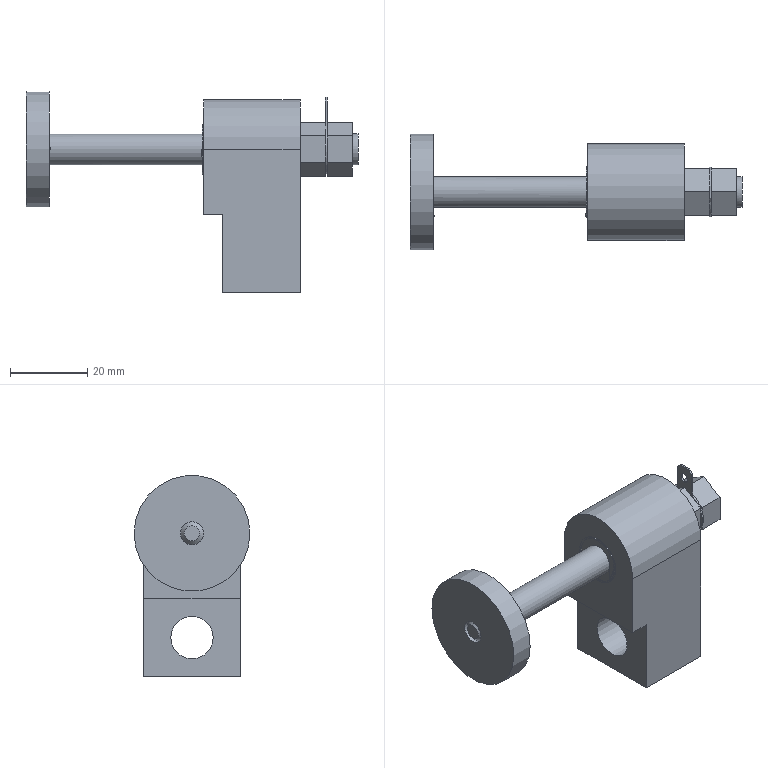Part | STEP file | PN_0059_id1358_x_t | 2 solids | 213 faces | box 86 x 30 x 52 mm | volume 33398 mm3 | plane 160 | cylinder 50 | spline 2 | cone 1 | commonest cylinder face diameters 8 x3 13 x3 1.416 x2 12.25 x2 0.67 x1 0.694 x1